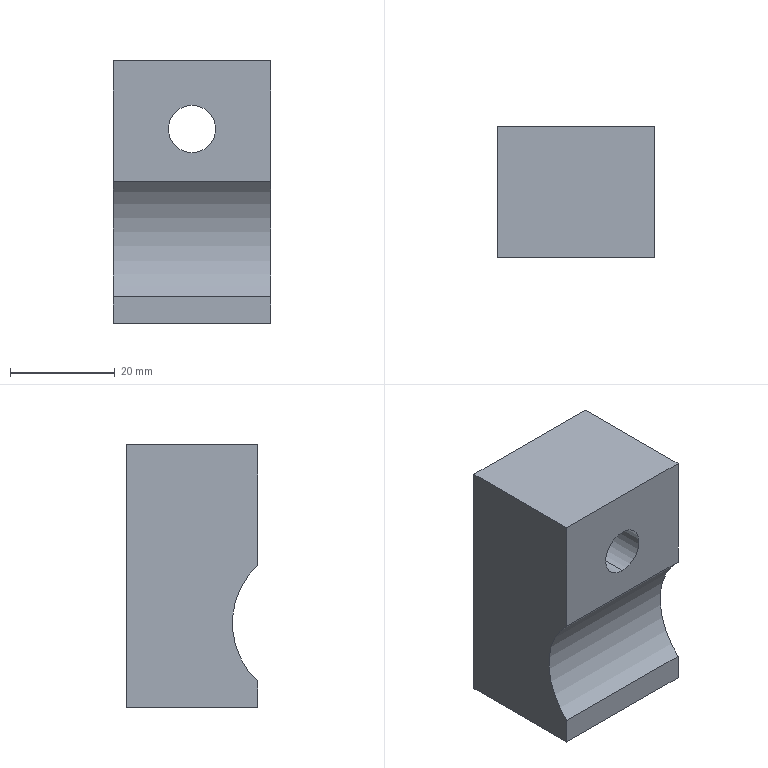Part | SolidWorks | features Extrusion 1, HoleWzd 1, ICE 1 | 1 solid | 10 faces | box 30 x 25 x 50 mm | volume 33718 mm3 | plane 7 | cylinder 3 | commonest cylinder face diameters 9 x2 30 x1
STEP:
#1=CARTESIAN_POINT('',(15.,0.,32.5));
#2=VERTEX_POINT('',#1);
#3=CARTESIAN_POINT('',(15.,0.,41.5));
#4=VERTEX_POINT('',#3);
#5=CARTESIAN_POINT('',(15.,0.,37.));
#6=DIRECTION('',(0.,1.,0.));
#7=DIRECTION('',(0.,0.,1.));
#8=AXIS2_PLACEMENT_3D('',#5,#6,#7);
#9=CIRCLE('',#8,4.5);
#10=EDGE_CURVE('',#2,#4,#9,.T.);
#11=ORIENTED_EDGE('',*,*,#10,.F.);
#12=CARTESIAN_POINT('',(15.,25.,32.5));
#13=VERTEX_POINT('',#12);
#14=CARTESIAN_POINT('',(15.,25.,32.5));
#15=DIRECTION('',(0.,1.,0.));
#16=VECTOR('',#15,1000.);
#17=LINE('',#14,#16);
#18=EDGE_CURVE('',#2,#13,#17,.T.);
#19=ORIENTED_EDGE('',*,*,#18,.T.);
#20=CARTESIAN_POINT('',(15.,25.,41.5));
#21=VERTEX_POINT('',#20);
#22=CARTESIAN_POINT('',(15.,25.,37.));
#23=DIRECTION('',(0.,1.,0.));
#24=DIRECTION('',(0.,0.,1.));
#25=AXIS2_PLACEMENT_3D('',#22,#23,#24);
#26=CIRCLE('',#25,4.5);
#27=EDGE_CURVE('',#13,#21,#26,.T.);
#28=ORIENTED_EDGE('',*,*,#27,.T.);
#29=CARTESIAN_POINT('',(15.,25.,41.5));
#30=DIRECTION('',(0.,1.,0.));
#31=VECTOR('',#30,1000.);
#32=LINE('',#29,#31);
#33=EDGE_CURVE('',#4,#21,#32,.T.);
#34=ORIENTED_EDGE('',*,*,#33,.F.);
#35=EDGE_LOOP('',(#11,#19,#28,#34));
#36=FACE_OUTER_BOUND('',#35,.T.);
#37=CARTESIAN_POINT('',(15.,25.,37.));
#38=DIRECTION('',(0.,1.,0.));
#39=DIRECTION('',(0.,0.,1.));
#40=AXIS2_PLACEMENT_3D('',#37,#38,#39);
#41=CYLINDRICAL_SURFACE('',#40,4.5);
#42=ADVANCED_FACE('',(#36),#41,.F.);
#43=CARTESIAN_POINT('',(0.,0.,27.));
#44=VERTEX_POINT('',#43);
#45=CARTESIAN_POINT('',(0.,0.,5.));
#46=VERTEX_POINT('',#45);
#47=CARTESIAN_POINT('',(0.,-10.198,16.));
#48=DIRECTION('',(-1.,0.,0.));
#49=DIRECTION('',(0.,0.,-1.));
#50=AXIS2_PLACEMENT_3D('',#47,#48,#49);
#51=CIRCLE('',#50,15.);
#52=EDGE_CURVE('',#44,#46,#51,.T.);
#53=ORIENTED_EDGE('',*,*,#52,.F.);
#54=CARTESIAN_POINT('',(0.,0.,50.));
#55=VERTEX_POINT('',#54);
#56=CARTESIAN_POINT('',(0.,0.,50.));
#57=DIRECTION('',(0.,0.,-1.));
#58=VECTOR('',#57,1000.);
#59=LINE('',#56,#58);
#60=EDGE_CURVE('',#55,#44,#59,.T.);
#61=ORIENTED_EDGE('',*,*,#60,.F.);
#62=CARTESIAN_POINT('',(0.,25.,50.));
#63=VERTEX_POINT('',#62);
#64=CARTESIAN_POINT('',(0.,0.,50.));
#65=DIRECTION('',(0.,-1.,0.));
#66=VECTOR('',#65,1000.);
#67=LINE('',#64,#66);
#68=EDGE_CURVE('',#63,#55,#67,.T.);
#69=ORIENTED_EDGE('',*,*,#68,.F.);
#70=CARTESIAN_POINT('',(0.,25.,0.));
#71=VERTEX_POINT('',#70);
#72=CARTESIAN_POINT('',(0.,25.,50.));
#73=DIRECTION('',(0.,0.,-1.));
#74=VECTOR('',#73,1000.);
#75=LINE('',#72,#74);
#76=EDGE_CURVE('',#63,#71,#75,.T.);
#77=ORIENTED_EDGE('',*,*,#76,.T.);
#78=CARTESIAN_POINT('',(0.,0.,0.));
#79=VERTEX_POINT('',#78);
#80=CARTESIAN_POINT('',(0.,0.,0.));
#81=DIRECTION('',(0.,-1.,0.));
#82=VECTOR('',#81,1000.);
#83=LINE('',#80,#82);
#84=EDGE_CURVE('',#71,#79,#83,.T.);
#85=ORIENTED_EDGE('',*,*,#84,.T.);
#86=CARTESIAN_POINT('',(0.,0.,50.));
#87=DIRECTION('',(0.,0.,-1.));
#88=VECTOR('',#87,1000.);
#89=LINE('',#86,#88);
#90=EDGE_CURVE('',#46,#79,#89,.T.);
#91=ORIENTED_EDGE('',*,*,#90,.F.);
#92=EDGE_LOOP('',(#53,#61,#69,#77,#85,#91));
#93=FACE_OUTER_BOUND('',#92,.T.);
#94=CARTESIAN_POINT('',(0.,0.,50.));
#95=DIRECTION('',(1.,0.,0.));
#96=DIRECTION('',(0.,0.,-1.));
#97=AXIS2_PLACEMENT_3D('',#94,#95,#96);
#98=PLANE('',#97);
#99=ADVANCED_FACE('',(#93),#98,.F.);
#100=CARTESIAN_POINT('',(15.,0.,37.));
#101=DIRECTION('',(0.,1.,0.));
#102=DIRECTION('',(0.,0.,1.));
#103=AXIS2_PLACEMENT_3D('',#100,#101,#102);
#104=CIRCLE('',#103,4.5);
#105=EDGE_CURVE('',#4,#2,#104,.T.);
#106=ORIENTED_EDGE('',*,*,#105,.T.);
#107=ORIENTED_EDGE('',*,*,#10,.T.);
#108=EDGE_LOOP('',(#106,#107));
#109=FACE_BOUND('',#108,.T.);
#110=CARTESIAN_POINT('',(30.,0.,27.));
#111=VERTEX_POINT('',#110);
#112=CARTESIAN_POINT('',(-65.,0.,27.));
#113=DIRECTION('',(1.,0.,0.));
#114=VECTOR('',#113,1000.);
#115=LINE('',#112,#114);
#116=EDGE_CURVE('',#44,#111,#115,.T.);
#117=ORIENTED_EDGE('',*,*,#116,.T.);
#118=CARTESIAN_POINT('',(30.,0.,50.));
#119=VERTEX_POINT('',#118);
#120=CARTESIAN_POINT('',(30.,0.,50.));
#121=DIRECTION('',(0.,0.,-1.));
#122=VECTOR('',#121,1000.);
#123=LINE('',#120,#122);
#124=EDGE_CURVE('',#119,#111,#123,.T.);
#125=ORIENTED_EDGE('',*,*,#124,.F.);
#126=CARTESIAN_POINT('',(0.,0.,50.));
#127=DIRECTION('',(1.,0.,0.));
#128=VECTOR('',#127,1000.);
#129=LINE('',#126,#128);
#130=EDGE_CURVE('',#55,#119,#129,.T.);
#131=ORIENTED_EDGE('',*,*,#130,.F.);
#132=ORIENTED_EDGE('',*,*,#60,.T.);
#133=EDGE_LOOP('',(#117,#125,#131,#132));
#134=FACE_OUTER_BOUND('',#133,.T.);
#135=CARTESIAN_POINT('',(0.,0.,50.));
#136=DIRECTION('',(0.,1.,0.));
#137=DIRECTION('',(0.,0.,1.));
#138=AXIS2_PLACEMENT_3D('',#135,#136,#137);
#139=PLANE('',#138);
#140=ADVANCED_FACE('',(#109,#134),#139,.F.);
#141=CARTESIAN_POINT('',(30.,0.,5.));
#142=VERTEX_POINT('',#141);
#143=CARTESIAN_POINT('',(-65.,0.,5.));
#144=DIRECTION('',(1.,0.,0.));
#145=VECTOR('',#144,1000.);
#146=LINE('',#143,#145);
#147=EDGE_CURVE('',#46,#142,#146,.T.);
#148=ORIENTED_EDGE('',*,*,#147,.F.);
#149=ORIENTED_EDGE('',*,*,#90,.T.);
#150=CARTESIAN_POINT('',(30.,0.,0.));
#151=VERTEX_POINT('',#150);
#152=CARTESIAN_POINT('',(0.,0.,0.));
#153=DIRECTION('',(1.,0.,0.));
#154=VECTOR('',#153,1000.);
#155=LINE('',#152,#154);
#156=EDGE_CURVE('',#79,#151,#155,.T.);
#157=ORIENTED_EDGE('',*,*,#156,.T.);
#158=CARTESIAN_POINT('',(30.,0.,50.));
#159=DIRECTION('',(0.,0.,-1.));
#160=VECTOR('',#159,1000.);
#161=LINE('',#158,#160);
#162=EDGE_CURVE('',#142,#151,#161,.T.);
#163=ORIENTED_EDGE('',*,*,#162,.F.);
#164=EDGE_LOOP('',(#148,#149,#157,#163));
#165=FACE_OUTER_BOUND('',#164,.T.);
#166=CARTESIAN_POINT('',(0.,0.,50.));
#167=DIRECTION('',(0.,1.,0.));
#168=DIRECTION('',(0.,0.,1.));
#169=AXIS2_PLACEMENT_3D('',#166,#167,#168);
#170=PLANE('',#169);
#171=ADVANCED_FACE('',(#165),#170,.F.);
#172=CARTESIAN_POINT('',(30.,-10.198,16.));
#173=DIRECTION('',(-1.,0.,0.));
#174=DIRECTION('',(0.,0.,1.));
#175=AXIS2_PLACEMENT_3D('',#172,#173,#174);
#176=CIRCLE('',#175,15.);
#177=EDGE_CURVE('',#111,#142,#176,.T.);
#178=ORIENTED_EDGE('',*,*,#177,.T.);
#179=ORIENTED_EDGE('',*,*,#162,.T.);
#180=CARTESIAN_POINT('',(30.,25.,0.));
#181=VERTEX_POINT('',#180);
#182=CARTESIAN_POINT('',(30.,0.,0.));
#183=DIRECTION('',(0.,1.,0.));
#184=VECTOR('',#183,1000.);
#185=LINE('',#182,#184);
#186=EDGE_CURVE('',#151,#181,#185,.T.);
#187=ORIENTED_EDGE('',*,*,#186,.T.);
#188=CARTESIAN_POINT('',(30.,25.,50.));
#189=VERTEX_POINT('',#188);
#190=CARTESIAN_POINT('',(30.,25.,50.));
#191=DIRECTION('',(0.,0.,-1.));
#192=VECTOR('',#191,1000.);
#193=LINE('',#190,#192);
#194=EDGE_CURVE('',#189,#181,#193,.T.);
#195=ORIENTED_EDGE('',*,*,#194,.F.);
#196=CARTESIAN_POINT('',(30.,0.,50.));
#197=DIRECTION('',(0.,1.,0.));
#198=VECTOR('',#197,1000.);
#199=LINE('',#196,#198);
#200=EDGE_CURVE('',#119,#189,#199,.T.);
#201=ORIENTED_EDGE('',*,*,#200,.F.);
#202=ORIENTED_EDGE('',*,*,#124,.T.);
#203=EDGE_LOOP('',(#178,#179,#187,#195,#201,#202));
#204=FACE_OUTER_BOUND('',#203,.T.);
#205=CARTESIAN_POINT('',(30.,0.,50.));
#206=DIRECTION('',(-1.,0.,0.));
#207=DIRECTION('',(0.,0.,1.));
#208=AXIS2_PLACEMENT_3D('',#205,#206,#207);
#209=PLANE('',#208);
#210=ADVANCED_FACE('',(#204),#209,.F.);
#211=CARTESIAN_POINT('',(15.,25.,37.));
#212=DIRECTION('',(0.,1.,0.));
#213=DIRECTION('',(0.,0.,1.));
#214=AXIS2_PLACEMENT_3D('',#211,#212,#213);
#215=CIRCLE('',#214,4.5);
#216=EDGE_CURVE('',#21,#13,#215,.T.);
#217=ORIENTED_EDGE('',*,*,#216,.F.);
#218=ORIENTED_EDGE('',*,*,#27,.F.);
#219=EDGE_LOOP('',(#217,#218));
#220=FACE_BOUND('',#219,.T.);
#221=CARTESIAN_POINT('',(0.,25.,0.));
#222=DIRECTION('',(-1.,0.,0.));
#223=VECTOR('',#222,1000.);
#224=LINE('',#221,#223);
#225=EDGE_CURVE('',#181,#71,#224,.T.);
#226=ORIENTED_EDGE('',*,*,#225,.T.);
#227=ORIENTED_EDGE('',*,*,#76,.F.);
#228=CARTESIAN_POINT('',(0.,25.,50.));
#229=DIRECTION('',(-1.,0.,0.));
#230=VECTOR('',#229,1000.);
#231=LINE('',#228,#230);
#232=EDGE_CURVE('',#189,#63,#231,.T.);
#233=ORIENTED_EDGE('',*,*,#232,.F.);
#234=ORIENTED_EDGE('',*,*,#194,.T.);
#235=EDGE_LOOP('',(#226,#227,#233,#234));
#236=FACE_OUTER_BOUND('',#235,.T.);
#237=CARTESIAN_POINT('',(0.,25.,50.));
#238=DIRECTION('',(0.,-1.,0.));
#239=DIRECTION('',(0.,0.,-1.));
#240=AXIS2_PLACEMENT_3D('',#237,#238,#239);
#241=PLANE('',#240);
#242=ADVANCED_FACE('',(#220,#236),#241,.F.);
#243=ORIENTED_EDGE('',*,*,#68,.T.);
#244=ORIENTED_EDGE('',*,*,#130,.T.);
#245=ORIENTED_EDGE('',*,*,#200,.T.);
#246=ORIENTED_EDGE('',*,*,#232,.T.);
#247=EDGE_LOOP('',(#243,#244,#245,#246));
#248=FACE_OUTER_BOUND('',#247,.T.);
#249=CARTESIAN_POINT('',(0.,25.,50.));
#250=DIRECTION('',(0.,0.,-1.));
#251=DIRECTION('',(-1.,0.,0.));
#252=AXIS2_PLACEMENT_3D('',#249,#250,#251);
#253=PLANE('',#252);
#254=ADVANCED_FACE('',(#248),#253,.F.);
#255=ORIENTED_EDGE('',*,*,#84,.F.);
#256=ORIENTED_EDGE('',*,*,#225,.F.);
#257=ORIENTED_EDGE('',*,*,#186,.F.);
#258=ORIENTED_EDGE('',*,*,#156,.F.);
#259=EDGE_LOOP('',(#255,#256,#257,#258));
#260=FACE_OUTER_BOUND('',#259,.T.);
#261=CARTESIAN_POINT('',(0.,25.,0.));
#262=DIRECTION('',(0.,0.,-1.));
#263=DIRECTION('',(-1.,0.,0.));
#264=AXIS2_PLACEMENT_3D('',#261,#262,#263);
#265=PLANE('',#264);
#266=ADVANCED_FACE('',(#260),#265,.T.);
#267=ORIENTED_EDGE('',*,*,#52,.T.);
#268=ORIENTED_EDGE('',*,*,#147,.T.);
#269=ORIENTED_EDGE('',*,*,#177,.F.);
#270=ORIENTED_EDGE('',*,*,#116,.F.);
#271=EDGE_LOOP('',(#267,#268,#269,#270));
#272=FACE_OUTER_BOUND('',#271,.T.);
#273=CARTESIAN_POINT('',(-65.,-10.198,16.));
#274=DIRECTION('',(1.,0.,0.));
#275=DIRECTION('',(0.,0.,-1.));
#276=AXIS2_PLACEMENT_3D('',#273,#274,#275);
#277=CYLINDRICAL_SURFACE('',#276,15.);
#278=ADVANCED_FACE('',(#272),#277,.F.);
#279=ORIENTED_EDGE('',*,*,#18,.F.);
#280=ORIENTED_EDGE('',*,*,#105,.F.);
#281=ORIENTED_EDGE('',*,*,#33,.T.);
#282=ORIENTED_EDGE('',*,*,#216,.T.);
#283=EDGE_LOOP('',(#279,#280,#281,#282));
#284=FACE_OUTER_BOUND('',#283,.T.);
#285=CARTESIAN_POINT('',(15.,25.,37.));
#286=DIRECTION('',(0.,1.,0.));
#287=DIRECTION('',(0.,0.,1.));
#288=AXIS2_PLACEMENT_3D('',#285,#286,#287);
#289=CYLINDRICAL_SURFACE('',#288,4.5);
#290=ADVANCED_FACE('',(#284),#289,.F.);
#291=CLOSED_SHELL('',(#42,#99,#140,#171,#210,#242,#254,#266,#278,#290));
#292=MANIFOLD_SOLID_BREP('',#291);
#293=CARTESIAN_POINT('',(0.,0.,0.));
#294=DIRECTION('',(0.,0.,1.));
#295=DIRECTION('',(1.,0.,0.));
#296=AXIS2_PLACEMENT_3D('',#293,#294,#295);
#297=(LENGTH_UNIT()NAMED_UNIT(*)SI_UNIT(.MILLI.,.METRE.));
#298=UNCERTAINTY_MEASURE_WITH_UNIT(LENGTH_MEASURE(0.00001),#297,'','');
#299=(NAMED_UNIT(*)PLANE_ANGLE_UNIT()SI_UNIT($,.RADIAN.));
#300=(NAMED_UNIT(*)SI_UNIT($,.STERADIAN.)SOLID_ANGLE_UNIT());
#301=(GEOMETRIC_REPRESENTATION_CONTEXT(3)GLOBAL_UNCERTAINTY_ASSIGNED_CONTEXT((#298))GLOBAL_UNIT_ASSIGNED_CONTEXT((#297,#299,#300))REPRESENTATION_CONTEXT('',''));
#302=ADVANCED_BREP_SHAPE_REPRESENTATION('',(#292,#296),#301);